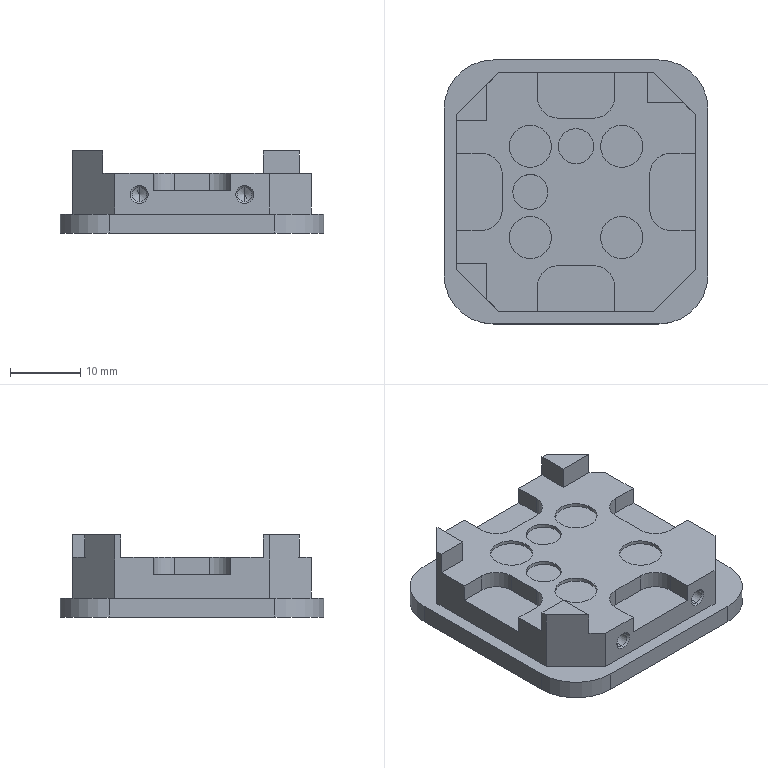Part | STEP file | CM-2-1-2.step-614.STEP | 1 solid | 100 faces | box 37.6 x 37.6 x 11.7 mm | volume 9215 mm3 | plane 46 | cylinder 34 | cone 20 | commonest cylinder face diameters 6 x16 2.05 x8 5 x4 14 x4 3.3 x2